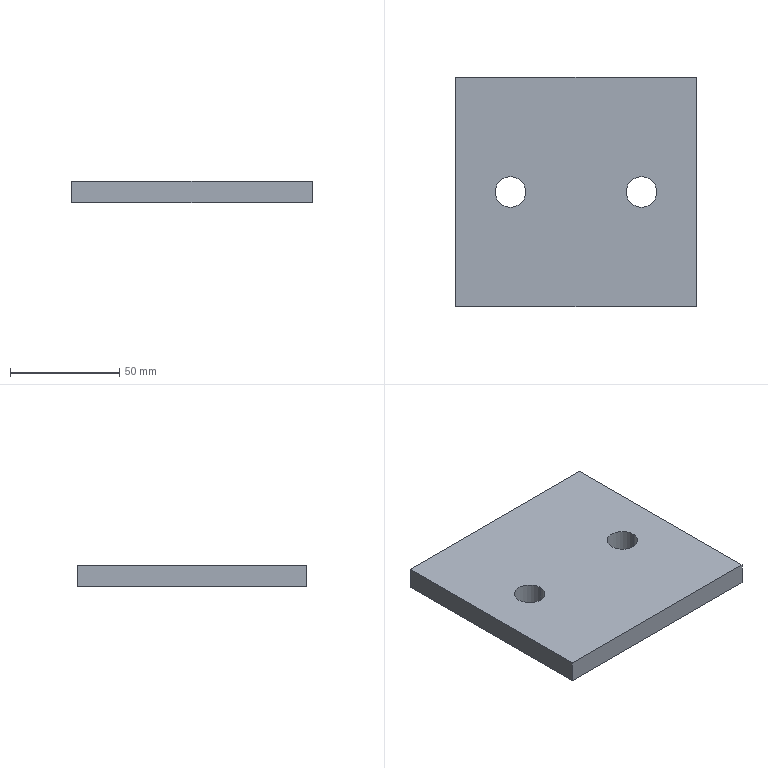Part | STEP file | 05-Connecting plate | 1 solid | 10 faces | box 110 x 105 x 10 mm | volume 112421 mm3 | plane 6 | cylinder 4 | commonest cylinder face diameters 14 x4
STEP:
#1=CARTESIAN_POINT('',(0.,0.,0.));
#2=DIRECTION('',(0.,0.,1.));
#3=DIRECTION('',(1.,0.,0.));
#4=AXIS2_PLACEMENT_3D('',#1,#2,#3);
#5=CARTESIAN_POINT('',(78.,-52.5,10.));
#6=VERTEX_POINT('',#5);
#7=CARTESIAN_POINT('',(78.,-52.5,0.));
#8=VERTEX_POINT('',#7);
#9=CARTESIAN_POINT('',(78.,-52.5,10.));
#10=DIRECTION('',(0.,0.,-1.));
#11=VECTOR('',#10,1.);
#12=LINE('',#9,#11);
#13=CARTESIAN_POINT('',(85.,-52.5,10.));
#14=DIRECTION('',(0.,0.,-1.));
#15=DIRECTION('',(-1.,0.,0.));
#16=AXIS2_PLACEMENT_3D('',#13,#14,#15);
#17=CYLINDRICAL_SURFACE('',#16,7.);
#18=CARTESIAN_POINT('',(6.283,0.));
#19=DIRECTION('',(0.,1.));
#20=VECTOR('',#19,1.);
#21=LINE('',#18,#20);
#22=(GEOMETRIC_REPRESENTATION_CONTEXT(2)PARAMETRIC_REPRESENTATION_CONTEXT()REPRESENTATION_CONTEXT('',''));
#23=DEFINITIONAL_REPRESENTATION('',(#21),#22);
#24=PCURVE('',#17,#23);
#25=CARTESIAN_POINT('',(85.,-52.5,10.));
#26=DIRECTION('',(0.,0.,-1.));
#27=DIRECTION('',(-1.,0.,0.));
#28=AXIS2_PLACEMENT_3D('',#25,#26,#27);
#29=CYLINDRICAL_SURFACE('',#28,7.);
#30=CARTESIAN_POINT('',(0.,0.));
#31=DIRECTION('',(0.,1.));
#32=VECTOR('',#31,1.);
#33=LINE('',#30,#32);
#34=(GEOMETRIC_REPRESENTATION_CONTEXT(2)PARAMETRIC_REPRESENTATION_CONTEXT()REPRESENTATION_CONTEXT('',''));
#35=DEFINITIONAL_REPRESENTATION('',(#33),#34);
#36=PCURVE('',#29,#35);
#37=SURFACE_CURVE('',#12,(#24,#36),.PCURVE_S1.);
#38=EDGE_CURVE('',#6,#8,#37,.T.);
#39=ORIENTED_EDGE('',*,*,#38,.T.);
#40=CARTESIAN_POINT('',(92.,-52.5,0.));
#41=VERTEX_POINT('',#40);
#42=CARTESIAN_POINT('',(85.,-52.5,0.));
#43=DIRECTION('',(0.,0.,1.));
#44=DIRECTION('',(1.,0.,0.));
#45=AXIS2_PLACEMENT_3D('',#42,#43,#44);
#46=CIRCLE('',#45,7.);
#47=CARTESIAN_POINT('',(9.425,10.));
#48=DIRECTION('',(-1.,0.));
#49=VECTOR('',#48,1.);
#50=LINE('',#47,#49);
#51=(GEOMETRIC_REPRESENTATION_CONTEXT(2)PARAMETRIC_REPRESENTATION_CONTEXT()REPRESENTATION_CONTEXT('',''));
#52=DEFINITIONAL_REPRESENTATION('',(#50),#51);
#53=PCURVE('',#17,#52);
#54=CARTESIAN_POINT('',(0.,0.,0.));
#55=DIRECTION('',(0.,0.,1.));
#56=DIRECTION('',(1.,0.,0.));
#57=AXIS2_PLACEMENT_3D('',#54,#55,#56);
#58=PLANE('',#57);
#59=CARTESIAN_POINT('',(85.,-52.5));
#60=DIRECTION('',(1.,0.));
#61=AXIS2_PLACEMENT_2D('',#59,#60);
#62=CIRCLE('',#61,7.);
#63=(GEOMETRIC_REPRESENTATION_CONTEXT(2)PARAMETRIC_REPRESENTATION_CONTEXT()REPRESENTATION_CONTEXT('',''));
#64=DEFINITIONAL_REPRESENTATION('',(#62),#63);
#65=PCURVE('',#58,#64);
#66=SURFACE_CURVE('',#46,(#53,#65),.PCURVE_S1.);
#67=EDGE_CURVE('',#8,#41,#66,.T.);
#68=ORIENTED_EDGE('',*,*,#67,.T.);
#69=CARTESIAN_POINT('',(92.,-52.5,10.));
#70=VERTEX_POINT('',#69);
#71=CARTESIAN_POINT('',(92.,-52.5,10.));
#72=DIRECTION('',(0.,0.,-1.));
#73=VECTOR('',#72,1.);
#74=LINE('',#71,#73);
#75=CARTESIAN_POINT('',(3.142,0.));
#76=DIRECTION('',(0.,1.));
#77=VECTOR('',#76,1.);
#78=LINE('',#75,#77);
#79=(GEOMETRIC_REPRESENTATION_CONTEXT(2)PARAMETRIC_REPRESENTATION_CONTEXT()REPRESENTATION_CONTEXT('',''));
#80=DEFINITIONAL_REPRESENTATION('',(#78),#79);
#81=PCURVE('',#17,#80);
#82=CARTESIAN_POINT('',(3.142,0.));
#83=DIRECTION('',(0.,1.));
#84=VECTOR('',#83,1.);
#85=LINE('',#82,#84);
#86=(GEOMETRIC_REPRESENTATION_CONTEXT(2)PARAMETRIC_REPRESENTATION_CONTEXT()REPRESENTATION_CONTEXT('',''));
#87=DEFINITIONAL_REPRESENTATION('',(#85),#86);
#88=PCURVE('',#29,#87);
#89=SURFACE_CURVE('',#74,(#81,#88),.PCURVE_S1.);
#90=EDGE_CURVE('',#70,#41,#89,.T.);
#91=ORIENTED_EDGE('',*,*,#90,.F.);
#92=CARTESIAN_POINT('',(85.,-52.5,10.));
#93=DIRECTION('',(0.,0.,1.));
#94=DIRECTION('',(1.,0.,0.));
#95=AXIS2_PLACEMENT_3D('',#92,#93,#94);
#96=CIRCLE('',#95,7.);
#97=CARTESIAN_POINT('',(9.425,0.));
#98=DIRECTION('',(-1.,0.));
#99=VECTOR('',#98,1.);
#100=LINE('',#97,#99);
#101=(GEOMETRIC_REPRESENTATION_CONTEXT(2)PARAMETRIC_REPRESENTATION_CONTEXT()REPRESENTATION_CONTEXT('',''));
#102=DEFINITIONAL_REPRESENTATION('',(#100),#101);
#103=PCURVE('',#17,#102);
#104=CARTESIAN_POINT('',(0.,0.,10.));
#105=DIRECTION('',(0.,0.,1.));
#106=DIRECTION('',(1.,0.,0.));
#107=AXIS2_PLACEMENT_3D('',#104,#105,#106);
#108=PLANE('',#107);
#109=CARTESIAN_POINT('',(85.,-52.5));
#110=DIRECTION('',(1.,0.));
#111=AXIS2_PLACEMENT_2D('',#109,#110);
#112=CIRCLE('',#111,7.);
#113=(GEOMETRIC_REPRESENTATION_CONTEXT(2)PARAMETRIC_REPRESENTATION_CONTEXT()REPRESENTATION_CONTEXT('',''));
#114=DEFINITIONAL_REPRESENTATION('',(#112),#113);
#115=PCURVE('',#108,#114);
#116=SURFACE_CURVE('',#96,(#103,#115),.PCURVE_S1.);
#117=EDGE_CURVE('',#6,#70,#116,.T.);
#118=ORIENTED_EDGE('',*,*,#117,.F.);
#119=EDGE_LOOP('',(#39,#68,#91,#118));
#120=FACE_BOUND('',#119,.F.);
#121=ADVANCED_FACE('',(#120),#17,.F.);
#122=CARTESIAN_POINT('',(18.,-52.5,10.));
#123=VERTEX_POINT('',#122);
#124=CARTESIAN_POINT('',(18.,-52.5,0.));
#125=VERTEX_POINT('',#124);
#126=CARTESIAN_POINT('',(18.,-52.5,10.));
#127=DIRECTION('',(0.,0.,-1.));
#128=VECTOR('',#127,1.);
#129=LINE('',#126,#128);
#130=CARTESIAN_POINT('',(25.,-52.5,10.));
#131=DIRECTION('',(0.,0.,-1.));
#132=DIRECTION('',(-1.,0.,0.));
#133=AXIS2_PLACEMENT_3D('',#130,#131,#132);
#134=CYLINDRICAL_SURFACE('',#133,7.);
#135=CARTESIAN_POINT('',(6.283,0.));
#136=DIRECTION('',(0.,1.));
#137=VECTOR('',#136,1.);
#138=LINE('',#135,#137);
#139=(GEOMETRIC_REPRESENTATION_CONTEXT(2)PARAMETRIC_REPRESENTATION_CONTEXT()REPRESENTATION_CONTEXT('',''));
#140=DEFINITIONAL_REPRESENTATION('',(#138),#139);
#141=PCURVE('',#134,#140);
#142=CARTESIAN_POINT('',(25.,-52.5,10.));
#143=DIRECTION('',(0.,0.,-1.));
#144=DIRECTION('',(-1.,0.,0.));
#145=AXIS2_PLACEMENT_3D('',#142,#143,#144);
#146=CYLINDRICAL_SURFACE('',#145,7.);
#147=CARTESIAN_POINT('',(0.,0.));
#148=DIRECTION('',(0.,1.));
#149=VECTOR('',#148,1.);
#150=LINE('',#147,#149);
#151=(GEOMETRIC_REPRESENTATION_CONTEXT(2)PARAMETRIC_REPRESENTATION_CONTEXT()REPRESENTATION_CONTEXT('',''));
#152=DEFINITIONAL_REPRESENTATION('',(#150),#151);
#153=PCURVE('',#146,#152);
#154=SURFACE_CURVE('',#129,(#141,#153),.PCURVE_S1.);
#155=EDGE_CURVE('',#123,#125,#154,.T.);
#156=ORIENTED_EDGE('',*,*,#155,.T.);
#157=CARTESIAN_POINT('',(32.,-52.5,0.));
#158=VERTEX_POINT('',#157);
#159=CARTESIAN_POINT('',(25.,-52.5,0.));
#160=DIRECTION('',(0.,0.,1.));
#161=DIRECTION('',(1.,0.,0.));
#162=AXIS2_PLACEMENT_3D('',#159,#160,#161);
#163=CIRCLE('',#162,7.);
#164=CARTESIAN_POINT('',(9.425,10.));
#165=DIRECTION('',(-1.,0.));
#166=VECTOR('',#165,1.);
#167=LINE('',#164,#166);
#168=(GEOMETRIC_REPRESENTATION_CONTEXT(2)PARAMETRIC_REPRESENTATION_CONTEXT()REPRESENTATION_CONTEXT('',''));
#169=DEFINITIONAL_REPRESENTATION('',(#167),#168);
#170=PCURVE('',#134,#169);
#171=CARTESIAN_POINT('',(25.,-52.5));
#172=DIRECTION('',(1.,0.));
#173=AXIS2_PLACEMENT_2D('',#171,#172);
#174=CIRCLE('',#173,7.);
#175=(GEOMETRIC_REPRESENTATION_CONTEXT(2)PARAMETRIC_REPRESENTATION_CONTEXT()REPRESENTATION_CONTEXT('',''));
#176=DEFINITIONAL_REPRESENTATION('',(#174),#175);
#177=PCURVE('',#58,#176);
#178=SURFACE_CURVE('',#163,(#170,#177),.PCURVE_S1.);
#179=EDGE_CURVE('',#125,#158,#178,.T.);
#180=ORIENTED_EDGE('',*,*,#179,.T.);
#181=CARTESIAN_POINT('',(32.,-52.5,10.));
#182=VERTEX_POINT('',#181);
#183=CARTESIAN_POINT('',(32.,-52.5,10.));
#184=DIRECTION('',(0.,0.,-1.));
#185=VECTOR('',#184,1.);
#186=LINE('',#183,#185);
#187=CARTESIAN_POINT('',(3.142,0.));
#188=DIRECTION('',(0.,1.));
#189=VECTOR('',#188,1.);
#190=LINE('',#187,#189);
#191=(GEOMETRIC_REPRESENTATION_CONTEXT(2)PARAMETRIC_REPRESENTATION_CONTEXT()REPRESENTATION_CONTEXT('',''));
#192=DEFINITIONAL_REPRESENTATION('',(#190),#191);
#193=PCURVE('',#134,#192);
#194=CARTESIAN_POINT('',(3.142,0.));
#195=DIRECTION('',(0.,1.));
#196=VECTOR('',#195,1.);
#197=LINE('',#194,#196);
#198=(GEOMETRIC_REPRESENTATION_CONTEXT(2)PARAMETRIC_REPRESENTATION_CONTEXT()REPRESENTATION_CONTEXT('',''));
#199=DEFINITIONAL_REPRESENTATION('',(#197),#198);
#200=PCURVE('',#146,#199);
#201=SURFACE_CURVE('',#186,(#193,#200),.PCURVE_S1.);
#202=EDGE_CURVE('',#182,#158,#201,.T.);
#203=ORIENTED_EDGE('',*,*,#202,.F.);
#204=CARTESIAN_POINT('',(25.,-52.5,10.));
#205=DIRECTION('',(0.,0.,1.));
#206=DIRECTION('',(1.,0.,0.));
#207=AXIS2_PLACEMENT_3D('',#204,#205,#206);
#208=CIRCLE('',#207,7.);
#209=CARTESIAN_POINT('',(9.425,0.));
#210=DIRECTION('',(-1.,0.));
#211=VECTOR('',#210,1.);
#212=LINE('',#209,#211);
#213=(GEOMETRIC_REPRESENTATION_CONTEXT(2)PARAMETRIC_REPRESENTATION_CONTEXT()REPRESENTATION_CONTEXT('',''));
#214=DEFINITIONAL_REPRESENTATION('',(#212),#213);
#215=PCURVE('',#134,#214);
#216=CARTESIAN_POINT('',(25.,-52.5));
#217=DIRECTION('',(1.,0.));
#218=AXIS2_PLACEMENT_2D('',#216,#217);
#219=CIRCLE('',#218,7.);
#220=(GEOMETRIC_REPRESENTATION_CONTEXT(2)PARAMETRIC_REPRESENTATION_CONTEXT()REPRESENTATION_CONTEXT('',''));
#221=DEFINITIONAL_REPRESENTATION('',(#219),#220);
#222=PCURVE('',#108,#221);
#223=SURFACE_CURVE('',#208,(#215,#222),.PCURVE_S1.);
#224=EDGE_CURVE('',#123,#182,#223,.T.);
#225=ORIENTED_EDGE('',*,*,#224,.F.);
#226=EDGE_LOOP('',(#156,#180,#203,#225));
#227=FACE_BOUND('',#226,.F.);
#228=ADVANCED_FACE('',(#227),#134,.F.);
#229=ORIENTED_EDGE('',*,*,#224,.F.);
#230=CARTESIAN_POINT('',(25.,-52.5,10.));
#231=DIRECTION('',(0.,0.,1.));
#232=DIRECTION('',(1.,0.,0.));
#233=AXIS2_PLACEMENT_3D('',#230,#231,#232);
#234=CIRCLE('',#233,7.);
#235=CARTESIAN_POINT('',(25.,-52.5));
#236=DIRECTION('',(1.,0.));
#237=AXIS2_PLACEMENT_2D('',#235,#236);
#238=CIRCLE('',#237,7.);
#239=(GEOMETRIC_REPRESENTATION_CONTEXT(2)PARAMETRIC_REPRESENTATION_CONTEXT()REPRESENTATION_CONTEXT('',''));
#240=DEFINITIONAL_REPRESENTATION('',(#238),#239);
#241=PCURVE('',#108,#240);
#242=CARTESIAN_POINT('',(3.142,0.));
#243=DIRECTION('',(-1.,0.));
#244=VECTOR('',#243,1.);
#245=LINE('',#242,#244);
#246=(GEOMETRIC_REPRESENTATION_CONTEXT(2)PARAMETRIC_REPRESENTATION_CONTEXT()REPRESENTATION_CONTEXT('',''));
#247=DEFINITIONAL_REPRESENTATION('',(#245),#246);
#248=PCURVE('',#146,#247);
#249=SURFACE_CURVE('',#234,(#241,#248),.PCURVE_S1.);
#250=EDGE_CURVE('',#182,#123,#249,.T.);
#251=ORIENTED_EDGE('',*,*,#250,.F.);
#252=EDGE_LOOP('',(#229,#251));
#253=FACE_BOUND('',#252,.T.);
#254=CARTESIAN_POINT('',(0.,0.,10.));
#255=VERTEX_POINT('',#254);
#256=CARTESIAN_POINT('',(0.,-105.,10.));
#257=VERTEX_POINT('',#256);
#258=CARTESIAN_POINT('',(0.,0.,10.));
#259=DIRECTION('',(0.,-1.,0.));
#260=VECTOR('',#259,1.);
#261=LINE('',#258,#260);
#262=CARTESIAN_POINT('',(0.,0.));
#263=DIRECTION('',(0.,-1.));
#264=VECTOR('',#263,1.);
#265=LINE('',#262,#264);
#266=(GEOMETRIC_REPRESENTATION_CONTEXT(2)PARAMETRIC_REPRESENTATION_CONTEXT()REPRESENTATION_CONTEXT('',''));
#267=DEFINITIONAL_REPRESENTATION('',(#265),#266);
#268=PCURVE('',#108,#267);
#269=CARTESIAN_POINT('',(0.,0.,10.));
#270=DIRECTION('',(1.,0.,0.));
#271=DIRECTION('',(0.,1.,0.));
#272=AXIS2_PLACEMENT_3D('',#269,#270,#271);
#273=PLANE('',#272);
#274=CARTESIAN_POINT('',(0.,0.));
#275=DIRECTION('',(-1.,0.));
#276=VECTOR('',#275,1.);
#277=LINE('',#274,#276);
#278=(GEOMETRIC_REPRESENTATION_CONTEXT(2)PARAMETRIC_REPRESENTATION_CONTEXT()REPRESENTATION_CONTEXT('',''));
#279=DEFINITIONAL_REPRESENTATION('',(#277),#278);
#280=PCURVE('',#273,#279);
#281=SURFACE_CURVE('',#261,(#268,#280),.PCURVE_S1.);
#282=EDGE_CURVE('',#255,#257,#281,.T.);
#283=ORIENTED_EDGE('',*,*,#282,.T.);
#284=CARTESIAN_POINT('',(110.,-105.,10.));
#285=VERTEX_POINT('',#284);
#286=CARTESIAN_POINT('',(0.,-105.,10.));
#287=DIRECTION('',(1.,0.,0.));
#288=VECTOR('',#287,1.);
#289=LINE('',#286,#288);
#290=CARTESIAN_POINT('',(0.,-105.));
#291=DIRECTION('',(1.,0.));
#292=VECTOR('',#291,1.);
#293=LINE('',#290,#292);
#294=(GEOMETRIC_REPRESENTATION_CONTEXT(2)PARAMETRIC_REPRESENTATION_CONTEXT()REPRESENTATION_CONTEXT('',''));
#295=DEFINITIONAL_REPRESENTATION('',(#293),#294);
#296=PCURVE('',#108,#295);
#297=CARTESIAN_POINT('',(0.,-105.,10.));
#298=DIRECTION('',(0.,1.,0.));
#299=DIRECTION('',(0.,0.,1.));
#300=AXIS2_PLACEMENT_3D('',#297,#298,#299);
#301=PLANE('',#300);
#302=CARTESIAN_POINT('',(0.,0.));
#303=DIRECTION('',(0.,1.));
#304=VECTOR('',#303,1.);
#305=LINE('',#302,#304);
#306=(GEOMETRIC_REPRESENTATION_CONTEXT(2)PARAMETRIC_REPRESENTATION_CONTEXT()REPRESENTATION_CONTEXT('',''));
#307=DEFINITIONAL_REPRESENTATION('',(#305),#306);
#308=PCURVE('',#301,#307);
#309=SURFACE_CURVE('',#289,(#296,#308),.PCURVE_S1.);
#310=EDGE_CURVE('',#257,#285,#309,.T.);
#311=ORIENTED_EDGE('',*,*,#310,.T.);
#312=CARTESIAN_POINT('',(110.,0.,10.));
#313=VERTEX_POINT('',#312);
#314=CARTESIAN_POINT('',(110.,0.,10.));
#315=DIRECTION('',(0.,1.,0.));
#316=VECTOR('',#315,1.);
#317=LINE('',#314,#316);
#318=CARTESIAN_POINT('',(110.,0.));
#319=DIRECTION('',(0.,1.));
#320=VECTOR('',#319,1.);
#321=LINE('',#318,#320);
#322=(GEOMETRIC_REPRESENTATION_CONTEXT(2)PARAMETRIC_REPRESENTATION_CONTEXT()REPRESENTATION_CONTEXT('',''));
#323=DEFINITIONAL_REPRESENTATION('',(#321),#322);
#324=PCURVE('',#108,#323);
#325=CARTESIAN_POINT('',(110.,0.,10.));
#326=DIRECTION('',(-1.,0.,0.));
#327=DIRECTION('',(0.,-1.,0.));
#328=AXIS2_PLACEMENT_3D('',#325,#326,#327);
#329=PLANE('',#328);
#330=CARTESIAN_POINT('',(0.,0.));
#331=DIRECTION('',(-1.,0.));
#332=VECTOR('',#331,1.);
#333=LINE('',#330,#332);
#334=(GEOMETRIC_REPRESENTATION_CONTEXT(2)PARAMETRIC_REPRESENTATION_CONTEXT()REPRESENTATION_CONTEXT('',''));
#335=DEFINITIONAL_REPRESENTATION('',(#333),#334);
#336=PCURVE('',#329,#335);
#337=SURFACE_CURVE('',#317,(#324,#336),.PCURVE_S1.);
#338=EDGE_CURVE('',#285,#313,#337,.T.);
#339=ORIENTED_EDGE('',*,*,#338,.T.);
#340=CARTESIAN_POINT('',(0.,0.,10.));
#341=DIRECTION('',(-1.,0.,0.));
#342=VECTOR('',#341,1.);
#343=LINE('',#340,#342);
#344=CARTESIAN_POINT('',(0.,0.));
#345=DIRECTION('',(-1.,0.));
#346=VECTOR('',#345,1.);
#347=LINE('',#344,#346);
#348=(GEOMETRIC_REPRESENTATION_CONTEXT(2)PARAMETRIC_REPRESENTATION_CONTEXT()REPRESENTATION_CONTEXT('',''));
#349=DEFINITIONAL_REPRESENTATION('',(#347),#348);
#350=PCURVE('',#108,#349);
#351=CARTESIAN_POINT('',(0.,0.,10.));
#352=DIRECTION('',(0.,-1.,0.));
#353=DIRECTION('',(0.,0.,-1.));
#354=AXIS2_PLACEMENT_3D('',#351,#352,#353);
#355=PLANE('',#354);
#356=CARTESIAN_POINT('',(0.,0.));
#357=DIRECTION('',(0.,-1.));
#358=VECTOR('',#357,1.);
#359=LINE('',#356,#358);
#360=(GEOMETRIC_REPRESENTATION_CONTEXT(2)PARAMETRIC_REPRESENTATION_CONTEXT()REPRESENTATION_CONTEXT('',''));
#361=DEFINITIONAL_REPRESENTATION('',(#359),#360);
#362=PCURVE('',#355,#361);
#363=SURFACE_CURVE('',#343,(#350,#362),.PCURVE_S1.);
#364=EDGE_CURVE('',#313,#255,#363,.T.);
#365=ORIENTED_EDGE('',*,*,#364,.T.);
#366=EDGE_LOOP('',(#283,#311,#339,#365));
#367=FACE_BOUND('',#366,.T.);
#368=ORIENTED_EDGE('',*,*,#117,.F.);
#369=CARTESIAN_POINT('',(85.,-52.5,10.));
#370=DIRECTION('',(0.,0.,1.));
#371=DIRECTION('',(1.,0.,0.));
#372=AXIS2_PLACEMENT_3D('',#369,#370,#371);
#373=CIRCLE('',#372,7.);
#374=CARTESIAN_POINT('',(85.,-52.5));
#375=DIRECTION('',(1.,0.));
#376=AXIS2_PLACEMENT_2D('',#374,#375);
#377=CIRCLE('',#376,7.);
#378=(GEOMETRIC_REPRESENTATION_CONTEXT(2)PARAMETRIC_REPRESENTATION_CONTEXT()REPRESENTATION_CONTEXT('',''));
#379=DEFINITIONAL_REPRESENTATION('',(#377),#378);
#380=PCURVE('',#108,#379);
#381=CARTESIAN_POINT('',(3.142,0.));
#382=DIRECTION('',(-1.,0.));
#383=VECTOR('',#382,1.);
#384=LINE('',#381,#383);
#385=(GEOMETRIC_REPRESENTATION_CONTEXT(2)PARAMETRIC_REPRESENTATION_CONTEXT()REPRESENTATION_CONTEXT('',''));
#386=DEFINITIONAL_REPRESENTATION('',(#384),#385);
#387=PCURVE('',#29,#386);
#388=SURFACE_CURVE('',#373,(#380,#387),.PCURVE_S1.);
#389=EDGE_CURVE('',#70,#6,#388,.T.);
#390=ORIENTED_EDGE('',*,*,#389,.F.);
#391=EDGE_LOOP('',(#368,#390));
#392=FACE_BOUND('',#391,.T.);
#393=ADVANCED_FACE('',(#253,#367,#392),#108,.T.);
#394=ORIENTED_EDGE('',*,*,#179,.T.);
#395=CARTESIAN_POINT('',(25.,-52.5,0.));
#396=DIRECTION('',(0.,0.,1.));
#397=DIRECTION('',(1.,0.,0.));
#398=AXIS2_PLACEMENT_3D('',#395,#396,#397);
#399=CIRCLE('',#398,7.);
#400=CARTESIAN_POINT('',(25.,-52.5));
#401=DIRECTION('',(1.,0.));
#402=AXIS2_PLACEMENT_2D('',#400,#401);
#403=CIRCLE('',#402,7.);
#404=(GEOMETRIC_REPRESENTATION_CONTEXT(2)PARAMETRIC_REPRESENTATION_CONTEXT()REPRESENTATION_CONTEXT('',''));
#405=DEFINITIONAL_REPRESENTATION('',(#403),#404);
#406=PCURVE('',#58,#405);
#407=CARTESIAN_POINT('',(3.142,10.));
#408=DIRECTION('',(-1.,0.));
#409=VECTOR('',#408,1.);
#410=LINE('',#407,#409);
#411=(GEOMETRIC_REPRESENTATION_CONTEXT(2)PARAMETRIC_REPRESENTATION_CONTEXT()REPRESENTATION_CONTEXT('',''));
#412=DEFINITIONAL_REPRESENTATION('',(#410),#411);
#413=PCURVE('',#146,#412);
#414=SURFACE_CURVE('',#399,(#406,#413),.PCURVE_S1.);
#415=EDGE_CURVE('',#158,#125,#414,.T.);
#416=ORIENTED_EDGE('',*,*,#415,.T.);
#417=EDGE_LOOP('',(#394,#416));
#418=FACE_BOUND('',#417,.T.);
#419=CARTESIAN_POINT('',(0.,0.,0.));
#420=VERTEX_POINT('',#419);
#421=CARTESIAN_POINT('',(0.,-105.,0.));
#422=VERTEX_POINT('',#421);
#423=CARTESIAN_POINT('',(0.,0.,0.));
#424=DIRECTION('',(0.,-1.,0.));
#425=VECTOR('',#424,1.);
#426=LINE('',#423,#425);
#427=CARTESIAN_POINT('',(0.,0.));
#428=DIRECTION('',(0.,-1.));
#429=VECTOR('',#428,1.);
#430=LINE('',#427,#429);
#431=(GEOMETRIC_REPRESENTATION_CONTEXT(2)PARAMETRIC_REPRESENTATION_CONTEXT()REPRESENTATION_CONTEXT('',''));
#432=DEFINITIONAL_REPRESENTATION('',(#430),#431);
#433=PCURVE('',#58,#432);
#434=CARTESIAN_POINT('',(0.,-10.));
#435=DIRECTION('',(-1.,0.));
#436=VECTOR('',#435,1.);
#437=LINE('',#434,#436);
#438=(GEOMETRIC_REPRESENTATION_CONTEXT(2)PARAMETRIC_REPRESENTATION_CONTEXT()REPRESENTATION_CONTEXT('',''));
#439=DEFINITIONAL_REPRESENTATION('',(#437),#438);
#440=PCURVE('',#273,#439);
#441=SURFACE_CURVE('',#426,(#433,#440),.PCURVE_S1.);
#442=EDGE_CURVE('',#420,#422,#441,.T.);
#443=ORIENTED_EDGE('',*,*,#442,.F.);
#444=CARTESIAN_POINT('',(110.,0.,0.));
#445=VERTEX_POINT('',#444);
#446=CARTESIAN_POINT('',(0.,0.,0.));
#447=DIRECTION('',(-1.,0.,0.));
#448=VECTOR('',#447,1.);
#449=LINE('',#446,#448);
#450=CARTESIAN_POINT('',(0.,0.));
#451=DIRECTION('',(-1.,0.));
#452=VECTOR('',#451,1.);
#453=LINE('',#450,#452);
#454=(GEOMETRIC_REPRESENTATION_CONTEXT(2)PARAMETRIC_REPRESENTATION_CONTEXT()REPRESENTATION_CONTEXT('',''));
#455=DEFINITIONAL_REPRESENTATION('',(#453),#454);
#456=PCURVE('',#58,#455);
#457=CARTESIAN_POINT('',(10.,0.));
#458=DIRECTION('',(0.,-1.));
#459=VECTOR('',#458,1.);
#460=LINE('',#457,#459);
#461=(GEOMETRIC_REPRESENTATION_CONTEXT(2)PARAMETRIC_REPRESENTATION_CONTEXT()REPRESENTATION_CONTEXT('',''));
#462=DEFINITIONAL_REPRESENTATION('',(#460),#461);
#463=PCURVE('',#355,#462);
#464=SURFACE_CURVE('',#449,(#456,#463),.PCURVE_S1.);
#465=EDGE_CURVE('',#445,#420,#464,.T.);
#466=ORIENTED_EDGE('',*,*,#465,.F.);
#467=CARTESIAN_POINT('',(110.,-105.,0.));
#468=VERTEX_POINT('',#467);
#469=CARTESIAN_POINT('',(110.,0.,0.));
#470=DIRECTION('',(0.,1.,0.));
#471=VECTOR('',#470,1.);
#472=LINE('',#469,#471);
#473=CARTESIAN_POINT('',(110.,0.));
#474=DIRECTION('',(0.,1.));
#475=VECTOR('',#474,1.);
#476=LINE('',#473,#475);
#477=(GEOMETRIC_REPRESENTATION_CONTEXT(2)PARAMETRIC_REPRESENTATION_CONTEXT()REPRESENTATION_CONTEXT('',''));
#478=DEFINITIONAL_REPRESENTATION('',(#476),#477);
#479=PCURVE('',#58,#478);
#480=CARTESIAN_POINT('',(0.,-10.));
#481=DIRECTION('',(-1.,0.));
#482=VECTOR('',#481,1.);
#483=LINE('',#480,#482);
#484=(GEOMETRIC_REPRESENTATION_CONTEXT(2)PARAMETRIC_REPRESENTATION_CONTEXT()REPRESENTATION_CONTEXT('',''));
#485=DEFINITIONAL_REPRESENTATION('',(#483),#484);
#486=PCURVE('',#329,#485);
#487=SURFACE_CURVE('',#472,(#479,#486),.PCURVE_S1.);
#488=EDGE_CURVE('',#468,#445,#487,.T.);
#489=ORIENTED_EDGE('',*,*,#488,.F.);
#490=CARTESIAN_POINT('',(0.,-105.,0.));
#491=DIRECTION('',(1.,0.,0.));
#492=VECTOR('',#491,1.);
#493=LINE('',#490,#492);
#494=CARTESIAN_POINT('',(0.,-105.));
#495=DIRECTION('',(1.,0.));
#496=VECTOR('',#495,1.);
#497=LINE('',#494,#496);
#498=(GEOMETRIC_REPRESENTATION_CONTEXT(2)PARAMETRIC_REPRESENTATION_CONTEXT()REPRESENTATION_CONTEXT('',''));
#499=DEFINITIONAL_REPRESENTATION('',(#497),#498);
#500=PCURVE('',#58,#499);
#501=CARTESIAN_POINT('',(-10.,0.));
#502=DIRECTION('',(0.,1.));
#503=VECTOR('',#502,1.);
#504=LINE('',#501,#503);
#505=(GEOMETRIC_REPRESENTATION_CONTEXT(2)PARAMETRIC_REPRESENTATION_CONTEXT()REPRESENTATION_CONTEXT('',''));
#506=DEFINITIONAL_REPRESENTATION('',(#504),#505);
#507=PCURVE('',#301,#506);
#508=SURFACE_CURVE('',#493,(#500,#507),.PCURVE_S1.);
#509=EDGE_CURVE('',#422,#468,#508,.T.);
#510=ORIENTED_EDGE('',*,*,#509,.F.);
#511=EDGE_LOOP('',(#443,#466,#489,#510));
#512=FACE_BOUND('',#511,.T.);
#513=ORIENTED_EDGE('',*,*,#67,.T.);
#514=CARTESIAN_POINT('',(85.,-52.5,0.));
#515=DIRECTION('',(0.,0.,1.));
#516=DIRECTION('',(1.,0.,0.));
#517=AXIS2_PLACEMENT_3D('',#514,#515,#516);
#518=CIRCLE('',#517,7.);
#519=CARTESIAN_POINT('',(85.,-52.5));
#520=DIRECTION('',(1.,0.));
#521=AXIS2_PLACEMENT_2D('',#519,#520);
#522=CIRCLE('',#521,7.);
#523=(GEOMETRIC_REPRESENTATION_CONTEXT(2)PARAMETRIC_REPRESENTATION_CONTEXT()REPRESENTATION_CONTEXT('',''));
#524=DEFINITIONAL_REPRESENTATION('',(#522),#523);
#525=PCURVE('',#58,#524);
#526=CARTESIAN_POINT('',(3.142,10.));
#527=DIRECTION('',(-1.,0.));
#528=VECTOR('',#527,1.);
#529=LINE('',#526,#528);
#530=(GEOMETRIC_REPRESENTATION_CONTEXT(2)PARAMETRIC_REPRESENTATION_CONTEXT()REPRESENTATION_CONTEXT('',''));
#531=DEFINITIONAL_REPRESENTATION('',(#529),#530);
#532=PCURVE('',#29,#531);
#533=SURFACE_CURVE('',#518,(#525,#532),.PCURVE_S1.);
#534=EDGE_CURVE('',#41,#8,#533,.T.);
#535=ORIENTED_EDGE('',*,*,#534,.T.);
#536=EDGE_LOOP('',(#513,#535));
#537=FACE_BOUND('',#536,.T.);
#538=ADVANCED_FACE('',(#418,#512,#537),#58,.F.);
#539=ORIENTED_EDGE('',*,*,#442,.T.);
#540=CARTESIAN_POINT('',(0.,-105.,10.));
#541=DIRECTION('',(0.,0.,-1.));
#542=VECTOR('',#541,1.);
#543=LINE('',#540,#542);
#544=CARTESIAN_POINT('',(-105.,0.));
#545=DIRECTION('',(0.,-1.));
#546=VECTOR('',#545,1.);
#547=LINE('',#544,#546);
#548=(GEOMETRIC_REPRESENTATION_CONTEXT(2)PARAMETRIC_REPRESENTATION_CONTEXT()REPRESENTATION_CONTEXT('',''));
#549=DEFINITIONAL_REPRESENTATION('',(#547),#548);
#550=PCURVE('',#273,#549);
#551=CARTESIAN_POINT('',(0.,0.));
#552=DIRECTION('',(-1.,0.));
#553=VECTOR('',#552,1.);
#554=LINE('',#551,#553);
#555=(GEOMETRIC_REPRESENTATION_CONTEXT(2)PARAMETRIC_REPRESENTATION_CONTEXT()REPRESENTATION_CONTEXT('',''));
#556=DEFINITIONAL_REPRESENTATION('',(#554),#555);
#557=PCURVE('',#301,#556);
#558=SURFACE_CURVE('',#543,(#550,#557),.PCURVE_S1.);
#559=EDGE_CURVE('',#257,#422,#558,.T.);
#560=ORIENTED_EDGE('',*,*,#559,.F.);
#561=ORIENTED_EDGE('',*,*,#282,.F.);
#562=CARTESIAN_POINT('',(0.,0.,10.));
#563=DIRECTION('',(0.,0.,-1.));
#564=VECTOR('',#563,1.);
#565=LINE('',#562,#564);
#566=CARTESIAN_POINT('',(0.,0.));
#567=DIRECTION('',(0.,-1.));
#568=VECTOR('',#567,1.);
#569=LINE('',#566,#568);
#570=(GEOMETRIC_REPRESENTATION_CONTEXT(2)PARAMETRIC_REPRESENTATION_CONTEXT()REPRESENTATION_CONTEXT('',''));
#571=DEFINITIONAL_REPRESENTATION('',(#569),#570);
#572=PCURVE('',#273,#571);
#573=CARTESIAN_POINT('',(0.,0.));
#574=DIRECTION('',(1.,0.));
#575=VECTOR('',#574,1.);
#576=LINE('',#573,#575);
#577=(GEOMETRIC_REPRESENTATION_CONTEXT(2)PARAMETRIC_REPRESENTATION_CONTEXT()REPRESENTATION_CONTEXT('',''));
#578=DEFINITIONAL_REPRESENTATION('',(#576),#577);
#579=PCURVE('',#355,#578);
#580=SURFACE_CURVE('',#565,(#572,#579),.PCURVE_S1.);
#581=EDGE_CURVE('',#255,#420,#580,.T.);
#582=ORIENTED_EDGE('',*,*,#581,.T.);
#583=EDGE_LOOP('',(#539,#560,#561,#582));
#584=FACE_BOUND('',#583,.T.);
#585=ADVANCED_FACE('',(#584),#273,.F.);
#586=ORIENTED_EDGE('',*,*,#509,.T.);
#587=CARTESIAN_POINT('',(110.,-105.,10.));
#588=DIRECTION('',(0.,0.,-1.));
#589=VECTOR('',#588,1.);
#590=LINE('',#587,#589);
#591=CARTESIAN_POINT('',(0.,110.));
#592=DIRECTION('',(-1.,0.));
#593=VECTOR('',#592,1.);
#594=LINE('',#591,#593);
#595=(GEOMETRIC_REPRESENTATION_CONTEXT(2)PARAMETRIC_REPRESENTATION_CONTEXT()REPRESENTATION_CONTEXT('',''));
#596=DEFINITIONAL_REPRESENTATION('',(#594),#595);
#597=PCURVE('',#301,#596);
#598=CARTESIAN_POINT('',(105.,0.));
#599=DIRECTION('',(0.,-1.));
#600=VECTOR('',#599,1.);
#601=LINE('',#598,#600);
#602=(GEOMETRIC_REPRESENTATION_CONTEXT(2)PARAMETRIC_REPRESENTATION_CONTEXT()REPRESENTATION_CONTEXT('',''));
#603=DEFINITIONAL_REPRESENTATION('',(#601),#602);
#604=PCURVE('',#329,#603);
#605=SURFACE_CURVE('',#590,(#597,#604),.PCURVE_S1.);
#606=EDGE_CURVE('',#285,#468,#605,.T.);
#607=ORIENTED_EDGE('',*,*,#606,.F.);
#608=ORIENTED_EDGE('',*,*,#310,.F.);
#609=ORIENTED_EDGE('',*,*,#559,.T.);
#610=EDGE_LOOP('',(#586,#607,#608,#609));
#611=FACE_BOUND('',#610,.T.);
#612=ADVANCED_FACE('',(#611),#301,.F.);
#613=ORIENTED_EDGE('',*,*,#488,.T.);
#614=CARTESIAN_POINT('',(110.,0.,10.));
#615=DIRECTION('',(0.,0.,-1.));
#616=VECTOR('',#615,1.);
#617=LINE('',#614,#616);
#618=CARTESIAN_POINT('',(0.,0.));
#619=DIRECTION('',(0.,-1.));
#620=VECTOR('',#619,1.);
#621=LINE('',#618,#620);
#622=(GEOMETRIC_REPRESENTATION_CONTEXT(2)PARAMETRIC_REPRESENTATION_CONTEXT()REPRESENTATION_CONTEXT('',''));
#623=DEFINITIONAL_REPRESENTATION('',(#621),#622);
#624=PCURVE('',#329,#623);
#625=CARTESIAN_POINT('',(0.,110.));
#626=DIRECTION('',(1.,0.));
#627=VECTOR('',#626,1.);
#628=LINE('',#625,#627);
#629=(GEOMETRIC_REPRESENTATION_CONTEXT(2)PARAMETRIC_REPRESENTATION_CONTEXT()REPRESENTATION_CONTEXT('',''));
#630=DEFINITIONAL_REPRESENTATION('',(#628),#629);
#631=PCURVE('',#355,#630);
#632=SURFACE_CURVE('',#617,(#624,#631),.PCURVE_S1.);
#633=EDGE_CURVE('',#313,#445,#632,.T.);
#634=ORIENTED_EDGE('',*,*,#633,.F.);
#635=ORIENTED_EDGE('',*,*,#338,.F.);
#636=ORIENTED_EDGE('',*,*,#606,.T.);
#637=EDGE_LOOP('',(#613,#634,#635,#636));
#638=FACE_BOUND('',#637,.T.);
#639=ADVANCED_FACE('',(#638),#329,.F.);
#640=ORIENTED_EDGE('',*,*,#465,.T.);
#641=ORIENTED_EDGE('',*,*,#581,.F.);
#642=ORIENTED_EDGE('',*,*,#364,.F.);
#643=ORIENTED_EDGE('',*,*,#633,.T.);
#644=EDGE_LOOP('',(#640,#641,#642,#643));
#645=FACE_BOUND('',#644,.T.);
#646=ADVANCED_FACE('',(#645),#355,.F.);
#647=ORIENTED_EDGE('',*,*,#415,.T.);
#648=ORIENTED_EDGE('',*,*,#155,.F.);
#649=ORIENTED_EDGE('',*,*,#250,.F.);
#650=ORIENTED_EDGE('',*,*,#202,.T.);
#651=EDGE_LOOP('',(#647,#648,#649,#650));
#652=FACE_BOUND('',#651,.F.);
#653=ADVANCED_FACE('',(#652),#146,.F.);
#654=ORIENTED_EDGE('',*,*,#534,.T.);
#655=ORIENTED_EDGE('',*,*,#38,.F.);
#656=ORIENTED_EDGE('',*,*,#389,.F.);
#657=ORIENTED_EDGE('',*,*,#90,.T.);
#658=EDGE_LOOP('',(#654,#655,#656,#657));
#659=FACE_BOUND('',#658,.F.);
#660=ADVANCED_FACE('',(#659),#29,.F.);
#661=CLOSED_SHELL('',(#121,#228,#393,#538,#585,#612,#639,#646,#653,#660));
#662=MANIFOLD_SOLID_BREP('',#661);
#663=(LENGTH_UNIT()NAMED_UNIT(*)SI_UNIT(.MILLI.,.METRE.));
#664=UNCERTAINTY_MEASURE_WITH_UNIT(LENGTH_MEASURE(0.0000001),#663,'','');
#665=(NAMED_UNIT(*)PLANE_ANGLE_UNIT()SI_UNIT($,.RADIAN.));
#666=(NAMED_UNIT(*)SI_UNIT($,.STERADIAN.)SOLID_ANGLE_UNIT());
#667=(GEOMETRIC_REPRESENTATION_CONTEXT(3)GLOBAL_UNCERTAINTY_ASSIGNED_CONTEXT((#664))GLOBAL_UNIT_ASSIGNED_CONTEXT((#663,#665,#666))REPRESENTATION_CONTEXT('',''));
#668=ADVANCED_BREP_SHAPE_REPRESENTATION('',(#4,#662),#667);